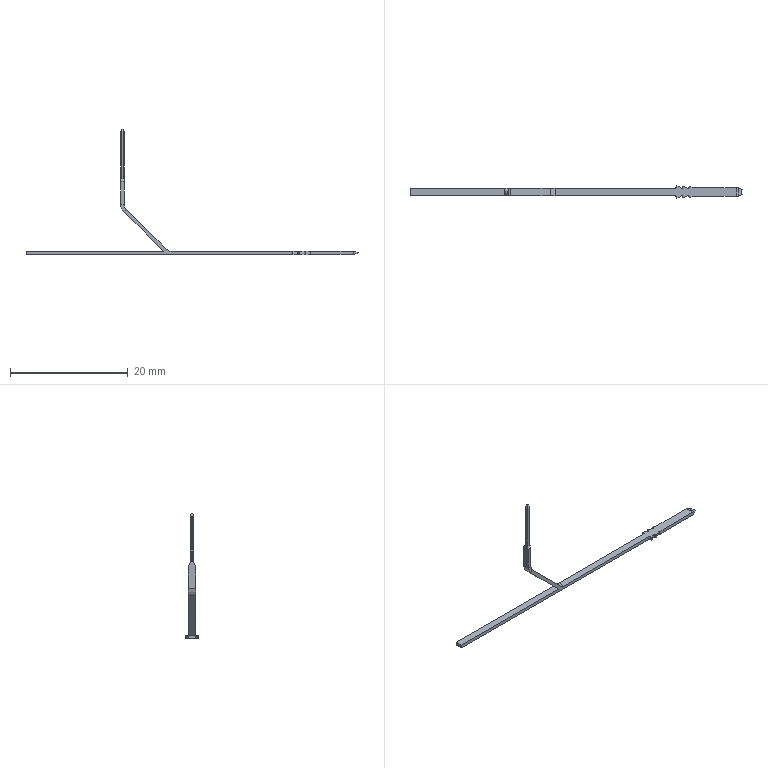Part | NX | features BREP 1 | 1 solid | 74 faces | box 56.403 x 2.1 x 21.3 mm | volume 56.28 mm3 | plane 42 | cylinder 32 | commonest cylinder face diameters 0.3 x12 0.2 x9 0.04 x4 0.025 x2 2 x2 2.4 x2